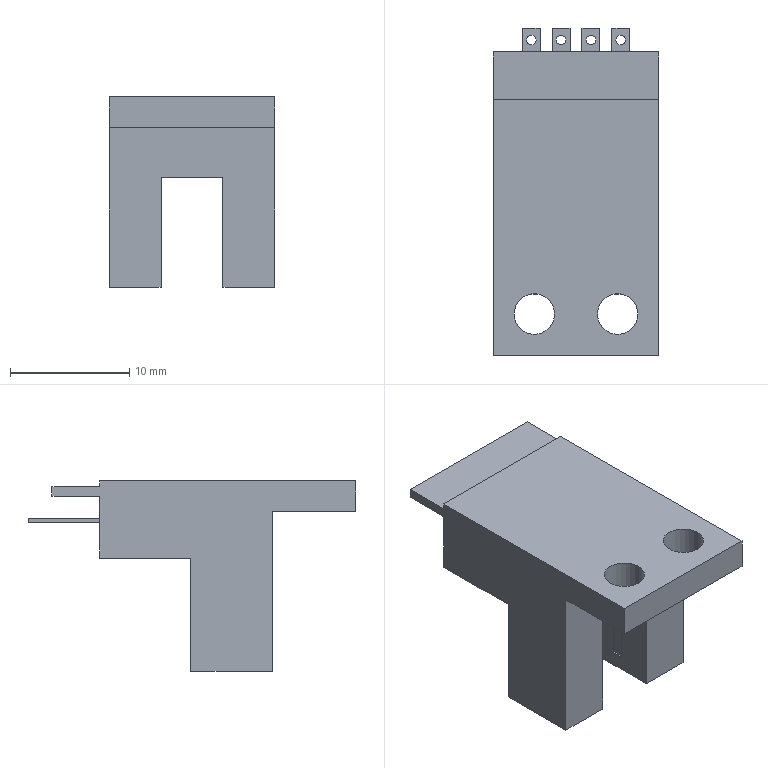Part | STEP file | 1 solid | 60 faces | box 13.9 x 27.5 x 16 mm | volume 2147 mm3 | plane 48 | cylinder 12 | commonest cylinder face diameters 0.8 x8 3.4 x4